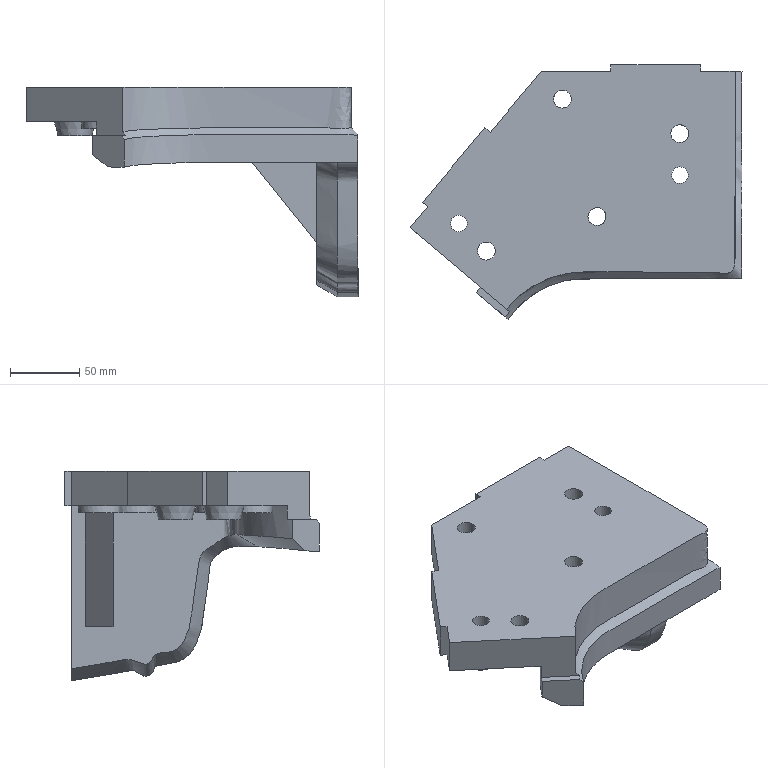Part | NX | features solid 2 | 1 solid | 48 faces | box 240.321 x 184.366 x 151.728 mm | volume 1269986 mm3 | plane 28 | cylinder 12 | spline 6 | cone 2 | commonest cylinder face diameters 13 x6 30 x4 12 x2